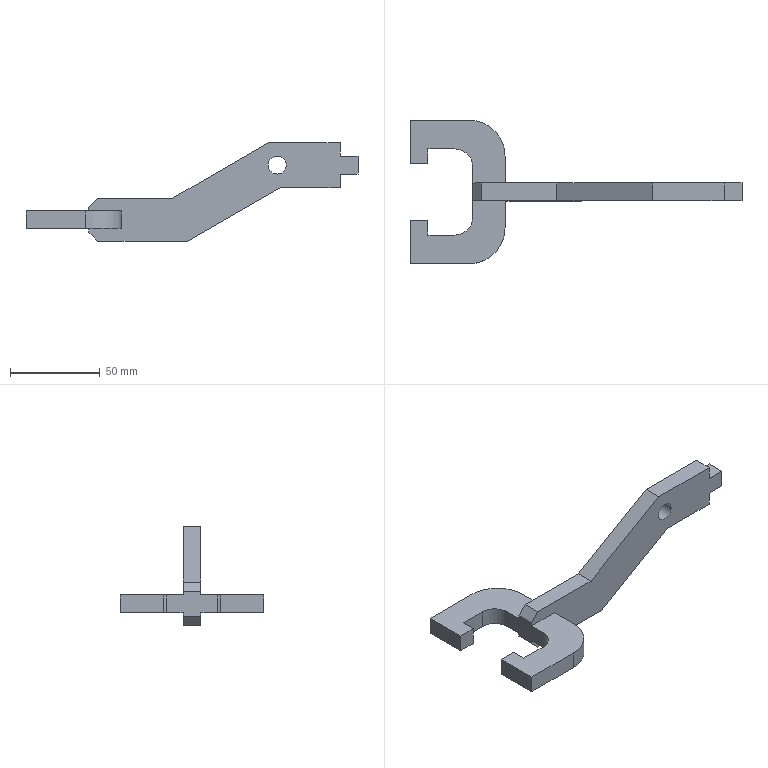Part | NX | features DATUM_CSYS 2, EXTRUDE 2, SKETCH 2, EXTRACT_DATUM_PLANE 1, LINKED_FACE 1 | 1 solid | 37 faces | box 185 x 80 x 55 mm | volume 60646 mm3 | plane 32 | cylinder 5 | commonest cylinder face diameters 20 x2 40 x2 10 x1
STEP:
#1=CARTESIAN_POINT('',(30.,5.,5.));
#2=VERTEX_POINT('',#1);
#3=CARTESIAN_POINT('',(30.,5.,7.));
#4=VERTEX_POINT('',#3);
#5=CARTESIAN_POINT('',(30.,5.,5.));
#6=DIRECTION('',(0.,0.,1.));
#7=VECTOR('',#6,1000.);
#8=LINE('',#5,#7);
#9=EDGE_CURVE('',#2,#4,#8,.T.);
#10=ORIENTED_EDGE('',*,*,#9,.F.);
#11=CARTESIAN_POINT('',(30.,14.,5.));
#12=VERTEX_POINT('',#11);
#13=CARTESIAN_POINT('',(30.,-14.,5.));
#14=DIRECTION('',(0.,1.,0.));
#15=VECTOR('',#14,1000.);
#16=LINE('',#13,#15);
#17=EDGE_CURVE('',#2,#12,#16,.T.);
#18=ORIENTED_EDGE('',*,*,#17,.T.);
#19=CARTESIAN_POINT('',(30.,14.,-5.));
#20=VERTEX_POINT('',#19);
#21=CARTESIAN_POINT('',(30.,14.,5.));
#22=DIRECTION('',(0.,0.,-1.));
#23=VECTOR('',#22,1000.);
#24=LINE('',#21,#23);
#25=EDGE_CURVE('',#12,#20,#24,.T.);
#26=ORIENTED_EDGE('',*,*,#25,.T.);
#27=CARTESIAN_POINT('',(30.,5.,-5.));
#28=VERTEX_POINT('',#27);
#29=CARTESIAN_POINT('',(30.,-14.,-5.));
#30=DIRECTION('',(0.,1.,0.));
#31=VECTOR('',#30,1000.);
#32=LINE('',#29,#31);
#33=EDGE_CURVE('',#28,#20,#32,.T.);
#34=ORIENTED_EDGE('',*,*,#33,.F.);
#35=CARTESIAN_POINT('',(30.,5.,-7.));
#36=VERTEX_POINT('',#35);
#37=CARTESIAN_POINT('',(30.,5.,-7.));
#38=DIRECTION('',(0.,0.,1.));
#39=VECTOR('',#38,1000.);
#40=LINE('',#37,#39);
#41=EDGE_CURVE('',#36,#28,#40,.T.);
#42=ORIENTED_EDGE('',*,*,#41,.F.);
#43=CARTESIAN_POINT('',(30.,-5.,-7.));
#44=VERTEX_POINT('',#43);
#45=CARTESIAN_POINT('',(30.,-5.,-7.));
#46=DIRECTION('',(0.,1.,0.));
#47=VECTOR('',#46,1000.);
#48=LINE('',#45,#47);
#49=EDGE_CURVE('',#44,#36,#48,.T.);
#50=ORIENTED_EDGE('',*,*,#49,.F.);
#51=CARTESIAN_POINT('',(30.,-5.,-5.));
#52=VERTEX_POINT('',#51);
#53=CARTESIAN_POINT('',(30.,-5.,-7.));
#54=DIRECTION('',(0.,0.,1.));
#55=VECTOR('',#54,1000.);
#56=LINE('',#53,#55);
#57=EDGE_CURVE('',#44,#52,#56,.T.);
#58=ORIENTED_EDGE('',*,*,#57,.T.);
#59=CARTESIAN_POINT('',(30.,-14.,-5.));
#60=VERTEX_POINT('',#59);
#61=CARTESIAN_POINT('',(30.,-14.,-5.));
#62=DIRECTION('',(0.,1.,0.));
#63=VECTOR('',#62,1000.);
#64=LINE('',#61,#63);
#65=EDGE_CURVE('',#60,#52,#64,.T.);
#66=ORIENTED_EDGE('',*,*,#65,.F.);
#67=CARTESIAN_POINT('',(30.,-14.,5.));
#68=VERTEX_POINT('',#67);
#69=CARTESIAN_POINT('',(30.,-14.,5.));
#70=DIRECTION('',(0.,0.,-1.));
#71=VECTOR('',#70,1000.);
#72=LINE('',#69,#71);
#73=EDGE_CURVE('',#68,#60,#72,.T.);
#74=ORIENTED_EDGE('',*,*,#73,.F.);
#75=CARTESIAN_POINT('',(30.,-5.,5.));
#76=VERTEX_POINT('',#75);
#77=CARTESIAN_POINT('',(30.,-14.,5.));
#78=DIRECTION('',(0.,1.,0.));
#79=VECTOR('',#78,1000.);
#80=LINE('',#77,#79);
#81=EDGE_CURVE('',#68,#76,#80,.T.);
#82=ORIENTED_EDGE('',*,*,#81,.T.);
#83=CARTESIAN_POINT('',(30.,-5.,7.));
#84=VERTEX_POINT('',#83);
#85=CARTESIAN_POINT('',(30.,-5.,5.));
#86=DIRECTION('',(0.,0.,1.));
#87=VECTOR('',#86,1000.);
#88=LINE('',#85,#87);
#89=EDGE_CURVE('',#76,#84,#88,.T.);
#90=ORIENTED_EDGE('',*,*,#89,.T.);
#91=CARTESIAN_POINT('',(30.,-5.,7.));
#92=DIRECTION('',(0.,1.,0.));
#93=VECTOR('',#92,1000.);
#94=LINE('',#91,#93);
#95=EDGE_CURVE('',#84,#4,#94,.T.);
#96=ORIENTED_EDGE('',*,*,#95,.T.);
#97=EDGE_LOOP('',(#10,#18,#26,#34,#42,#50,#58,#66,#74,#82,#90,#96));
#98=FACE_BOUND('',#97,.T.);
#99=CARTESIAN_POINT('',(30.,-5.,5.));
#100=DIRECTION('',(-1.,0.,0.));
#101=DIRECTION('',(0.,0.,1.));
#102=AXIS2_PLACEMENT_3D('',#99,#100,#101);
#103=PLANE('',#102);
#104=ADVANCED_FACE('',(#98),#103,.T.);
#105=CARTESIAN_POINT('',(35.016,5.,12.016));
#106=VERTEX_POINT('',#105);
#107=CARTESIAN_POINT('',(30.,5.,7.));
#108=DIRECTION('',(0.7071,0.,0.7071));
#109=VECTOR('',#108,1000.);
#110=LINE('',#107,#109);
#111=EDGE_CURVE('',#4,#106,#110,.T.);
#112=ORIENTED_EDGE('',*,*,#111,.F.);
#113=ORIENTED_EDGE('',*,*,#95,.F.);
#114=CARTESIAN_POINT('',(35.016,-5.,12.016));
#115=VERTEX_POINT('',#114);
#116=CARTESIAN_POINT('',(30.,-5.,7.));
#117=DIRECTION('',(0.7071,0.,0.7071));
#118=VECTOR('',#117,1000.);
#119=LINE('',#116,#118);
#120=EDGE_CURVE('',#84,#115,#119,.T.);
#121=ORIENTED_EDGE('',*,*,#120,.T.);
#122=CARTESIAN_POINT('',(35.016,-5.,12.016));
#123=DIRECTION('',(0.,1.,0.));
#124=VECTOR('',#123,1000.);
#125=LINE('',#122,#124);
#126=EDGE_CURVE('',#115,#106,#125,.T.);
#127=ORIENTED_EDGE('',*,*,#126,.T.);
#128=EDGE_LOOP('',(#112,#113,#121,#127));
#129=FACE_BOUND('',#128,.T.);
#130=CARTESIAN_POINT('',(30.,-5.,7.));
#131=DIRECTION('',(-0.7071,0.,0.7071));
#132=DIRECTION('',(0.7071,0.,0.7071));
#133=AXIS2_PLACEMENT_3D('',#130,#131,#132);
#134=PLANE('',#133);
#135=ADVANCED_FACE('',(#129),#134,.T.);
#136=CARTESIAN_POINT('',(76.823,5.,12.146));
#137=VERTEX_POINT('',#136);
#138=CARTESIAN_POINT('',(35.016,5.,12.016));
#139=DIRECTION('',(1.,0.,0.003125));
#140=VECTOR('',#139,1000.);
#141=LINE('',#138,#140);
#142=EDGE_CURVE('',#106,#137,#141,.T.);
#143=ORIENTED_EDGE('',*,*,#142,.F.);
#144=ORIENTED_EDGE('',*,*,#126,.F.);
#145=CARTESIAN_POINT('',(76.823,-5.,12.146));
#146=VERTEX_POINT('',#145);
#147=CARTESIAN_POINT('',(35.016,-5.,12.016));
#148=DIRECTION('',(1.,0.,0.003125));
#149=VECTOR('',#148,1000.);
#150=LINE('',#147,#149);
#151=EDGE_CURVE('',#115,#146,#150,.T.);
#152=ORIENTED_EDGE('',*,*,#151,.T.);
#153=CARTESIAN_POINT('',(76.823,-5.,12.146));
#154=DIRECTION('',(0.,1.,0.));
#155=VECTOR('',#154,1000.);
#156=LINE('',#153,#155);
#157=EDGE_CURVE('',#146,#137,#156,.T.);
#158=ORIENTED_EDGE('',*,*,#157,.T.);
#159=EDGE_LOOP('',(#143,#144,#152,#158));
#160=FACE_BOUND('',#159,.T.);
#161=CARTESIAN_POINT('',(35.016,-5.,12.016));
#162=DIRECTION('',(-0.003125,0.,1.));
#163=DIRECTION('',(1.,0.,0.003125));
#164=AXIS2_PLACEMENT_3D('',#161,#162,#163);
#165=PLANE('',#164);
#166=ADVANCED_FACE('',(#160),#165,.T.);
#167=CARTESIAN_POINT('',(130.263,5.,43.));
#168=VERTEX_POINT('',#167);
#169=CARTESIAN_POINT('',(76.823,5.,12.146));
#170=DIRECTION('',(0.866,0.,0.5));
#171=VECTOR('',#170,1000.);
#172=LINE('',#169,#171);
#173=EDGE_CURVE('',#137,#168,#172,.T.);
#174=ORIENTED_EDGE('',*,*,#173,.F.);
#175=ORIENTED_EDGE('',*,*,#157,.F.);
#176=CARTESIAN_POINT('',(130.263,-5.,43.));
#177=VERTEX_POINT('',#176);
#178=CARTESIAN_POINT('',(76.823,-5.,12.146));
#179=DIRECTION('',(0.866,0.,0.5));
#180=VECTOR('',#179,1000.);
#181=LINE('',#178,#180);
#182=EDGE_CURVE('',#146,#177,#181,.T.);
#183=ORIENTED_EDGE('',*,*,#182,.T.);
#184=CARTESIAN_POINT('',(130.263,-5.,43.));
#185=DIRECTION('',(0.,1.,0.));
#186=VECTOR('',#185,1000.);
#187=LINE('',#184,#186);
#188=EDGE_CURVE('',#177,#168,#187,.T.);
#189=ORIENTED_EDGE('',*,*,#188,.T.);
#190=EDGE_LOOP('',(#174,#175,#183,#189));
#191=FACE_BOUND('',#190,.T.);
#192=CARTESIAN_POINT('',(76.823,-5.,12.146));
#193=DIRECTION('',(-0.5,0.,0.866));
#194=DIRECTION('',(0.866,0.,0.5));
#195=AXIS2_PLACEMENT_3D('',#192,#193,#194);
#196=PLANE('',#195);
#197=ADVANCED_FACE('',(#191),#196,.T.);
#198=CARTESIAN_POINT('',(170.,5.,43.));
#199=VERTEX_POINT('',#198);
#200=CARTESIAN_POINT('',(130.263,5.,43.));
#201=DIRECTION('',(1.,0.,0.));
#202=VECTOR('',#201,1000.);
#203=LINE('',#200,#202);
#204=EDGE_CURVE('',#168,#199,#203,.T.);
#205=ORIENTED_EDGE('',*,*,#204,.F.);
#206=ORIENTED_EDGE('',*,*,#188,.F.);
#207=CARTESIAN_POINT('',(170.,-5.,43.));
#208=VERTEX_POINT('',#207);
#209=CARTESIAN_POINT('',(130.263,-5.,43.));
#210=DIRECTION('',(1.,0.,0.));
#211=VECTOR('',#210,1000.);
#212=LINE('',#209,#211);
#213=EDGE_CURVE('',#177,#208,#212,.T.);
#214=ORIENTED_EDGE('',*,*,#213,.T.);
#215=CARTESIAN_POINT('',(170.,-5.,43.));
#216=DIRECTION('',(0.,1.,0.));
#217=VECTOR('',#216,1000.);
#218=LINE('',#215,#217);
#219=EDGE_CURVE('',#208,#199,#218,.T.);
#220=ORIENTED_EDGE('',*,*,#219,.T.);
#221=EDGE_LOOP('',(#205,#206,#214,#220));
#222=FACE_BOUND('',#221,.T.);
#223=CARTESIAN_POINT('',(130.263,-5.,43.));
#224=DIRECTION('',(0.,0.,1.));
#225=DIRECTION('',(1.,0.,0.));
#226=AXIS2_PLACEMENT_3D('',#223,#224,#225);
#227=PLANE('',#226);
#228=ADVANCED_FACE('',(#222),#227,.T.);
#229=CARTESIAN_POINT('',(170.,5.,35.5));
#230=VERTEX_POINT('',#229);
#231=CARTESIAN_POINT('',(170.,5.,43.));
#232=DIRECTION('',(0.,0.,-1.));
#233=VECTOR('',#232,1000.);
#234=LINE('',#231,#233);
#235=EDGE_CURVE('',#199,#230,#234,.T.);
#236=ORIENTED_EDGE('',*,*,#235,.F.);
#237=ORIENTED_EDGE('',*,*,#219,.F.);
#238=CARTESIAN_POINT('',(170.,-5.,35.5));
#239=VERTEX_POINT('',#238);
#240=CARTESIAN_POINT('',(170.,-5.,43.));
#241=DIRECTION('',(0.,0.,-1.));
#242=VECTOR('',#241,1000.);
#243=LINE('',#240,#242);
#244=EDGE_CURVE('',#208,#239,#243,.T.);
#245=ORIENTED_EDGE('',*,*,#244,.T.);
#246=CARTESIAN_POINT('',(170.,-5.,35.5));
#247=DIRECTION('',(0.,1.,0.));
#248=VECTOR('',#247,1000.);
#249=LINE('',#246,#248);
#250=EDGE_CURVE('',#239,#230,#249,.T.);
#251=ORIENTED_EDGE('',*,*,#250,.T.);
#252=EDGE_LOOP('',(#236,#237,#245,#251));
#253=FACE_BOUND('',#252,.T.);
#254=CARTESIAN_POINT('',(170.,-5.,43.));
#255=DIRECTION('',(1.,0.,0.));
#256=DIRECTION('',(0.,0.,-1.));
#257=AXIS2_PLACEMENT_3D('',#254,#255,#256);
#258=PLANE('',#257);
#259=ADVANCED_FACE('',(#253),#258,.T.);
#260=CARTESIAN_POINT('',(180.,5.,35.5));
#261=VERTEX_POINT('',#260);
#262=CARTESIAN_POINT('',(170.,5.,35.5));
#263=DIRECTION('',(1.,0.,0.));
#264=VECTOR('',#263,1000.);
#265=LINE('',#262,#264);
#266=EDGE_CURVE('',#230,#261,#265,.T.);
#267=ORIENTED_EDGE('',*,*,#266,.F.);
#268=ORIENTED_EDGE('',*,*,#250,.F.);
#269=CARTESIAN_POINT('',(180.,-5.,35.5));
#270=VERTEX_POINT('',#269);
#271=CARTESIAN_POINT('',(170.,-5.,35.5));
#272=DIRECTION('',(1.,0.,0.));
#273=VECTOR('',#272,1000.);
#274=LINE('',#271,#273);
#275=EDGE_CURVE('',#239,#270,#274,.T.);
#276=ORIENTED_EDGE('',*,*,#275,.T.);
#277=CARTESIAN_POINT('',(180.,-5.,35.5));
#278=DIRECTION('',(0.,1.,0.));
#279=VECTOR('',#278,1000.);
#280=LINE('',#277,#279);
#281=EDGE_CURVE('',#270,#261,#280,.T.);
#282=ORIENTED_EDGE('',*,*,#281,.T.);
#283=EDGE_LOOP('',(#267,#268,#276,#282));
#284=FACE_BOUND('',#283,.T.);
#285=CARTESIAN_POINT('',(170.,-5.,35.5));
#286=DIRECTION('',(0.,0.,1.));
#287=DIRECTION('',(1.,0.,0.));
#288=AXIS2_PLACEMENT_3D('',#285,#286,#287);
#289=PLANE('',#288);
#290=ADVANCED_FACE('',(#284),#289,.T.);
#291=CARTESIAN_POINT('',(180.,5.,25.5));
#292=VERTEX_POINT('',#291);
#293=CARTESIAN_POINT('',(180.,5.,35.5));
#294=DIRECTION('',(0.,0.,-1.));
#295=VECTOR('',#294,1000.);
#296=LINE('',#293,#295);
#297=EDGE_CURVE('',#261,#292,#296,.T.);
#298=ORIENTED_EDGE('',*,*,#297,.F.);
#299=ORIENTED_EDGE('',*,*,#281,.F.);
#300=CARTESIAN_POINT('',(180.,-5.,25.5));
#301=VERTEX_POINT('',#300);
#302=CARTESIAN_POINT('',(180.,-5.,35.5));
#303=DIRECTION('',(0.,0.,-1.));
#304=VECTOR('',#303,1000.);
#305=LINE('',#302,#304);
#306=EDGE_CURVE('',#270,#301,#305,.T.);
#307=ORIENTED_EDGE('',*,*,#306,.T.);
#308=CARTESIAN_POINT('',(180.,-5.,25.5));
#309=DIRECTION('',(0.,1.,0.));
#310=VECTOR('',#309,1000.);
#311=LINE('',#308,#310);
#312=EDGE_CURVE('',#301,#292,#311,.T.);
#313=ORIENTED_EDGE('',*,*,#312,.T.);
#314=EDGE_LOOP('',(#298,#299,#307,#313));
#315=FACE_BOUND('',#314,.T.);
#316=CARTESIAN_POINT('',(180.,-5.,35.5));
#317=DIRECTION('',(1.,0.,0.));
#318=DIRECTION('',(0.,0.,-1.));
#319=AXIS2_PLACEMENT_3D('',#316,#317,#318);
#320=PLANE('',#319);
#321=ADVANCED_FACE('',(#315),#320,.T.);
#322=CARTESIAN_POINT('',(170.,5.,25.5));
#323=VERTEX_POINT('',#322);
#324=CARTESIAN_POINT('',(180.,5.,25.5));
#325=DIRECTION('',(-1.,0.,0.));
#326=VECTOR('',#325,1000.);
#327=LINE('',#324,#326);
#328=EDGE_CURVE('',#292,#323,#327,.T.);
#329=ORIENTED_EDGE('',*,*,#328,.F.);
#330=ORIENTED_EDGE('',*,*,#312,.F.);
#331=CARTESIAN_POINT('',(170.,-5.,25.5));
#332=VERTEX_POINT('',#331);
#333=CARTESIAN_POINT('',(180.,-5.,25.5));
#334=DIRECTION('',(-1.,0.,0.));
#335=VECTOR('',#334,1000.);
#336=LINE('',#333,#335);
#337=EDGE_CURVE('',#301,#332,#336,.T.);
#338=ORIENTED_EDGE('',*,*,#337,.T.);
#339=CARTESIAN_POINT('',(170.,-5.,25.5));
#340=DIRECTION('',(0.,1.,0.));
#341=VECTOR('',#340,1000.);
#342=LINE('',#339,#341);
#343=EDGE_CURVE('',#332,#323,#342,.T.);
#344=ORIENTED_EDGE('',*,*,#343,.T.);
#345=EDGE_LOOP('',(#329,#330,#338,#344));
#346=FACE_BOUND('',#345,.T.);
#347=CARTESIAN_POINT('',(180.,-5.,25.5));
#348=DIRECTION('',(0.,0.,-1.));
#349=DIRECTION('',(-1.,0.,0.));
#350=AXIS2_PLACEMENT_3D('',#347,#348,#349);
#351=PLANE('',#350);
#352=ADVANCED_FACE('',(#346),#351,.T.);
#353=CARTESIAN_POINT('',(170.,5.,18.));
#354=VERTEX_POINT('',#353);
#355=CARTESIAN_POINT('',(170.,5.,25.5));
#356=DIRECTION('',(0.,0.,-1.));
#357=VECTOR('',#356,1000.);
#358=LINE('',#355,#357);
#359=EDGE_CURVE('',#323,#354,#358,.T.);
#360=ORIENTED_EDGE('',*,*,#359,.F.);
#361=ORIENTED_EDGE('',*,*,#343,.F.);
#362=CARTESIAN_POINT('',(170.,-5.,18.));
#363=VERTEX_POINT('',#362);
#364=CARTESIAN_POINT('',(170.,-5.,25.5));
#365=DIRECTION('',(0.,0.,-1.));
#366=VECTOR('',#365,1000.);
#367=LINE('',#364,#366);
#368=EDGE_CURVE('',#332,#363,#367,.T.);
#369=ORIENTED_EDGE('',*,*,#368,.T.);
#370=CARTESIAN_POINT('',(170.,-5.,18.));
#371=DIRECTION('',(0.,1.,0.));
#372=VECTOR('',#371,1000.);
#373=LINE('',#370,#372);
#374=EDGE_CURVE('',#363,#354,#373,.T.);
#375=ORIENTED_EDGE('',*,*,#374,.T.);
#376=EDGE_LOOP('',(#360,#361,#369,#375));
#377=FACE_BOUND('',#376,.T.);
#378=CARTESIAN_POINT('',(170.,-5.,25.5));
#379=DIRECTION('',(1.,0.,0.));
#380=DIRECTION('',(0.,0.,-1.));
#381=AXIS2_PLACEMENT_3D('',#378,#379,#380);
#382=PLANE('',#381);
#383=ADVANCED_FACE('',(#377),#382,.T.);
#384=CARTESIAN_POINT('',(136.962,5.,18.));
#385=VERTEX_POINT('',#384);
#386=CARTESIAN_POINT('',(170.,5.,18.));
#387=DIRECTION('',(-1.,0.,0.));
#388=VECTOR('',#387,1000.);
#389=LINE('',#386,#388);
#390=EDGE_CURVE('',#354,#385,#389,.T.);
#391=ORIENTED_EDGE('',*,*,#390,.F.);
#392=ORIENTED_EDGE('',*,*,#374,.F.);
#393=CARTESIAN_POINT('',(136.962,-5.,18.));
#394=VERTEX_POINT('',#393);
#395=CARTESIAN_POINT('',(170.,-5.,18.));
#396=DIRECTION('',(-1.,0.,0.));
#397=VECTOR('',#396,1000.);
#398=LINE('',#395,#397);
#399=EDGE_CURVE('',#363,#394,#398,.T.);
#400=ORIENTED_EDGE('',*,*,#399,.T.);
#401=CARTESIAN_POINT('',(136.962,-5.,18.));
#402=DIRECTION('',(0.,1.,0.));
#403=VECTOR('',#402,1000.);
#404=LINE('',#401,#403);
#405=EDGE_CURVE('',#394,#385,#404,.T.);
#406=ORIENTED_EDGE('',*,*,#405,.T.);
#407=EDGE_LOOP('',(#391,#392,#400,#406));
#408=FACE_BOUND('',#407,.T.);
#409=CARTESIAN_POINT('',(170.,-5.,18.));
#410=DIRECTION('',(0.,0.,-1.));
#411=DIRECTION('',(-1.,0.,0.));
#412=AXIS2_PLACEMENT_3D('',#409,#410,#411);
#413=PLANE('',#412);
#414=ADVANCED_FACE('',(#408),#413,.T.);
#415=CARTESIAN_POINT('',(85.,5.,-12.));
#416=VERTEX_POINT('',#415);
#417=CARTESIAN_POINT('',(136.962,5.,18.));
#418=DIRECTION('',(-0.866,0.,-0.5));
#419=VECTOR('',#418,1000.);
#420=LINE('',#417,#419);
#421=EDGE_CURVE('',#385,#416,#420,.T.);
#422=ORIENTED_EDGE('',*,*,#421,.F.);
#423=ORIENTED_EDGE('',*,*,#405,.F.);
#424=CARTESIAN_POINT('',(85.,-5.,-12.));
#425=VERTEX_POINT('',#424);
#426=CARTESIAN_POINT('',(136.962,-5.,18.));
#427=DIRECTION('',(-0.866,0.,-0.5));
#428=VECTOR('',#427,1000.);
#429=LINE('',#426,#428);
#430=EDGE_CURVE('',#394,#425,#429,.T.);
#431=ORIENTED_EDGE('',*,*,#430,.T.);
#432=CARTESIAN_POINT('',(85.,-5.,-12.));
#433=DIRECTION('',(0.,1.,0.));
#434=VECTOR('',#433,1000.);
#435=LINE('',#432,#434);
#436=EDGE_CURVE('',#425,#416,#435,.T.);
#437=ORIENTED_EDGE('',*,*,#436,.T.);
#438=EDGE_LOOP('',(#422,#423,#431,#437));
#439=FACE_BOUND('',#438,.T.);
#440=CARTESIAN_POINT('',(136.962,-5.,18.));
#441=DIRECTION('',(0.5,0.,-0.866));
#442=DIRECTION('',(-0.866,0.,-0.5));
#443=AXIS2_PLACEMENT_3D('',#440,#441,#442);
#444=PLANE('',#443);
#445=ADVANCED_FACE('',(#439),#444,.T.);
#446=CARTESIAN_POINT('',(35.,5.,-12.));
#447=VERTEX_POINT('',#446);
#448=CARTESIAN_POINT('',(85.,5.,-12.));
#449=DIRECTION('',(-1.,0.,0.));
#450=VECTOR('',#449,1000.);
#451=LINE('',#448,#450);
#452=EDGE_CURVE('',#416,#447,#451,.T.);
#453=ORIENTED_EDGE('',*,*,#452,.F.);
#454=ORIENTED_EDGE('',*,*,#436,.F.);
#455=CARTESIAN_POINT('',(35.,-5.,-12.));
#456=VERTEX_POINT('',#455);
#457=CARTESIAN_POINT('',(85.,-5.,-12.));
#458=DIRECTION('',(-1.,0.,0.));
#459=VECTOR('',#458,1000.);
#460=LINE('',#457,#459);
#461=EDGE_CURVE('',#425,#456,#460,.T.);
#462=ORIENTED_EDGE('',*,*,#461,.T.);
#463=CARTESIAN_POINT('',(35.,-5.,-12.));
#464=DIRECTION('',(0.,1.,0.));
#465=VECTOR('',#464,1000.);
#466=LINE('',#463,#465);
#467=EDGE_CURVE('',#456,#447,#466,.T.);
#468=ORIENTED_EDGE('',*,*,#467,.T.);
#469=EDGE_LOOP('',(#453,#454,#462,#468));
#470=FACE_BOUND('',#469,.T.);
#471=CARTESIAN_POINT('',(85.,-5.,-12.));
#472=DIRECTION('',(0.,0.,-1.));
#473=DIRECTION('',(-1.,0.,0.));
#474=AXIS2_PLACEMENT_3D('',#471,#472,#473);
#475=PLANE('',#474);
#476=ADVANCED_FACE('',(#470),#475,.T.);
#477=CARTESIAN_POINT('',(35.,5.,-12.));
#478=DIRECTION('',(-0.7071,0.,0.7071));
#479=VECTOR('',#478,1000.);
#480=LINE('',#477,#479);
#481=EDGE_CURVE('',#447,#36,#480,.T.);
#482=ORIENTED_EDGE('',*,*,#481,.F.);
#483=ORIENTED_EDGE('',*,*,#467,.F.);
#484=CARTESIAN_POINT('',(35.,-5.,-12.));
#485=DIRECTION('',(-0.7071,0.,0.7071));
#486=VECTOR('',#485,1000.);
#487=LINE('',#484,#486);
#488=EDGE_CURVE('',#456,#44,#487,.T.);
#489=ORIENTED_EDGE('',*,*,#488,.T.);
#490=ORIENTED_EDGE('',*,*,#49,.T.);
#491=EDGE_LOOP('',(#482,#483,#489,#490));
#492=FACE_BOUND('',#491,.T.);
#493=CARTESIAN_POINT('',(35.,-5.,-12.));
#494=DIRECTION('',(-0.7071,0.,-0.7071));
#495=DIRECTION('',(-0.7071,0.,0.7071));
#496=AXIS2_PLACEMENT_3D('',#493,#494,#495);
#497=PLANE('',#496);
#498=ADVANCED_FACE('',(#492),#497,.T.);
#499=CARTESIAN_POINT('',(135.,5.,25.5));
#500=VERTEX_POINT('',#499);
#501=CARTESIAN_POINT('',(135.,5.,30.5));
#502=DIRECTION('',(0.,-1.,0.));
#503=DIRECTION('',(0.,0.,-1.));
#504=AXIS2_PLACEMENT_3D('',#501,#502,#503);
#505=CIRCLE('',#504,5.);
#506=EDGE_CURVE('',#500,#500,#505,.T.);
#507=ORIENTED_EDGE('',*,*,#506,.F.);
#508=EDGE_LOOP('',(#507));
#509=FACE_BOUND('',#508,.T.);
#510=CARTESIAN_POINT('',(135.,-5.,35.5));
#511=VERTEX_POINT('',#510);
#512=CARTESIAN_POINT('',(135.,-5.,30.5));
#513=DIRECTION('',(0.,-1.,0.));
#514=DIRECTION('',(0.,0.,1.));
#515=AXIS2_PLACEMENT_3D('',#512,#513,#514);
#516=CIRCLE('',#515,5.);
#517=EDGE_CURVE('',#511,#511,#516,.T.);
#518=ORIENTED_EDGE('',*,*,#517,.T.);
#519=EDGE_LOOP('',(#518));
#520=FACE_BOUND('',#519,.T.);
#521=CARTESIAN_POINT('',(135.,-5.,30.5));
#522=DIRECTION('',(0.,1.,0.));
#523=DIRECTION('',(0.,0.,1.));
#524=AXIS2_PLACEMENT_3D('',#521,#522,#523);
#525=CYLINDRICAL_SURFACE('',#524,5.);
#526=ADVANCED_FACE('',(#509,#520),#525,.F.);
#527=ORIENTED_EDGE('',*,*,#57,.F.);
#528=ORIENTED_EDGE('',*,*,#488,.F.);
#529=ORIENTED_EDGE('',*,*,#461,.F.);
#530=ORIENTED_EDGE('',*,*,#430,.F.);
#531=ORIENTED_EDGE('',*,*,#399,.F.);
#532=ORIENTED_EDGE('',*,*,#368,.F.);
#533=ORIENTED_EDGE('',*,*,#337,.F.);
#534=ORIENTED_EDGE('',*,*,#306,.F.);
#535=ORIENTED_EDGE('',*,*,#275,.F.);
#536=ORIENTED_EDGE('',*,*,#244,.F.);
#537=ORIENTED_EDGE('',*,*,#213,.F.);
#538=ORIENTED_EDGE('',*,*,#182,.F.);
#539=ORIENTED_EDGE('',*,*,#151,.F.);
#540=ORIENTED_EDGE('',*,*,#120,.F.);
#541=ORIENTED_EDGE('',*,*,#89,.F.);
#542=CARTESIAN_POINT('',(48.,-5.,5.));
#543=VERTEX_POINT('',#542);
#544=CARTESIAN_POINT('',(48.,-5.,5.));
#545=DIRECTION('',(-1.,0.,0.));
#546=VECTOR('',#545,1000.);
#547=LINE('',#544,#546);
#548=EDGE_CURVE('',#543,#76,#547,.T.);
#549=ORIENTED_EDGE('',*,*,#548,.F.);
#550=CARTESIAN_POINT('',(48.,-5.,-5.));
#551=VERTEX_POINT('',#550);
#552=CARTESIAN_POINT('',(48.,-5.,-5.));
#553=DIRECTION('',(0.,0.,1.));
#554=VECTOR('',#553,1000.);
#555=LINE('',#552,#554);
#556=EDGE_CURVE('',#551,#543,#555,.T.);
#557=ORIENTED_EDGE('',*,*,#556,.F.);
#558=CARTESIAN_POINT('',(30.,-5.,-5.));
#559=DIRECTION('',(1.,0.,0.));
#560=VECTOR('',#559,1000.);
#561=LINE('',#558,#560);
#562=EDGE_CURVE('',#52,#551,#561,.T.);
#563=ORIENTED_EDGE('',*,*,#562,.F.);
#564=EDGE_LOOP('',(#527,#528,#529,#530,#531,#532,#533,#534,#535,#536,#537,#538,#539,#540,#541,#549,#557,#563));
#565=FACE_BOUND('',#564,.T.);
#566=ORIENTED_EDGE('',*,*,#517,.F.);
#567=EDGE_LOOP('',(#566));
#568=FACE_BOUND('',#567,.T.);
#569=CARTESIAN_POINT('',(135.,-5.,30.5));
#570=DIRECTION('',(0.,-1.,0.));
#571=DIRECTION('',(0.,0.,-1.));
#572=AXIS2_PLACEMENT_3D('',#569,#570,#571);
#573=PLANE('',#572);
#574=ADVANCED_FACE('',(#565,#568),#573,.T.);
#575=ORIENTED_EDGE('',*,*,#41,.T.);
#576=CARTESIAN_POINT('',(48.,5.,-5.));
#577=VERTEX_POINT('',#576);
#578=CARTESIAN_POINT('',(30.,5.,-5.));
#579=DIRECTION('',(1.,0.,0.));
#580=VECTOR('',#579,1000.);
#581=LINE('',#578,#580);
#582=EDGE_CURVE('',#28,#577,#581,.T.);
#583=ORIENTED_EDGE('',*,*,#582,.T.);
#584=CARTESIAN_POINT('',(48.,5.,5.));
#585=VERTEX_POINT('',#584);
#586=CARTESIAN_POINT('',(48.,5.,-5.));
#587=DIRECTION('',(0.,0.,1.));
#588=VECTOR('',#587,1000.);
#589=LINE('',#586,#588);
#590=EDGE_CURVE('',#577,#585,#589,.T.);
#591=ORIENTED_EDGE('',*,*,#590,.T.);
#592=CARTESIAN_POINT('',(48.,5.,5.));
#593=DIRECTION('',(-1.,0.,0.));
#594=VECTOR('',#593,1000.);
#595=LINE('',#592,#594);
#596=EDGE_CURVE('',#585,#2,#595,.T.);
#597=ORIENTED_EDGE('',*,*,#596,.T.);
#598=ORIENTED_EDGE('',*,*,#9,.T.);
#599=ORIENTED_EDGE('',*,*,#111,.T.);
#600=ORIENTED_EDGE('',*,*,#142,.T.);
#601=ORIENTED_EDGE('',*,*,#173,.T.);
#602=ORIENTED_EDGE('',*,*,#204,.T.);
#603=ORIENTED_EDGE('',*,*,#235,.T.);
#604=ORIENTED_EDGE('',*,*,#266,.T.);
#605=ORIENTED_EDGE('',*,*,#297,.T.);
#606=ORIENTED_EDGE('',*,*,#328,.T.);
#607=ORIENTED_EDGE('',*,*,#359,.T.);
#608=ORIENTED_EDGE('',*,*,#390,.T.);
#609=ORIENTED_EDGE('',*,*,#421,.T.);
#610=ORIENTED_EDGE('',*,*,#452,.T.);
#611=ORIENTED_EDGE('',*,*,#481,.T.);
#612=EDGE_LOOP('',(#575,#583,#591,#597,#598,#599,#600,#601,#602,#603,#604,#605,#606,#607,#608,#609,#610,#611));
#613=FACE_BOUND('',#612,.T.);
#614=ORIENTED_EDGE('',*,*,#506,.T.);
#615=EDGE_LOOP('',(#614));
#616=FACE_BOUND('',#615,.T.);
#617=CARTESIAN_POINT('',(135.,5.,30.5));
#618=DIRECTION('',(0.,-1.,0.));
#619=DIRECTION('',(0.,0.,-1.));
#620=AXIS2_PLACEMENT_3D('',#617,#618,#619);
#621=PLANE('',#620);
#622=ADVANCED_FACE('',(#613,#616),#621,.F.);
#623=ORIENTED_EDGE('',*,*,#65,.T.);
#624=ORIENTED_EDGE('',*,*,#562,.T.);
#625=CARTESIAN_POINT('',(48.,-20.,-5.));
#626=VERTEX_POINT('',#625);
#627=CARTESIAN_POINT('',(48.,20.,-5.));
#628=DIRECTION('',(0.,-1.,0.));
#629=VECTOR('',#628,1000.);
#630=LINE('',#627,#629);
#631=EDGE_CURVE('',#551,#626,#630,.T.);
#632=ORIENTED_EDGE('',*,*,#631,.T.);
#633=CARTESIAN_POINT('',(28.,-40.,-5.));
#634=VERTEX_POINT('',#633);
#635=CARTESIAN_POINT('',(28.,-20.,-5.));
#636=DIRECTION('',(0.,0.,-1.));
#637=DIRECTION('',(1.,0.,0.));
#638=AXIS2_PLACEMENT_3D('',#635,#636,#637);
#639=CIRCLE('',#638,20.);
#640=EDGE_CURVE('',#626,#634,#639,.T.);
#641=ORIENTED_EDGE('',*,*,#640,.T.);
#642=CARTESIAN_POINT('',(-5.,-40.,-5.));
#643=VERTEX_POINT('',#642);
#644=CARTESIAN_POINT('',(-3.,-40.,-5.));
#645=DIRECTION('',(-1.,0.,0.));
#646=VECTOR('',#645,1000.);
#647=LINE('',#644,#646);
#648=EDGE_CURVE('',#634,#643,#647,.T.);
#649=ORIENTED_EDGE('',*,*,#648,.T.);
#650=CARTESIAN_POINT('',(-5.,-16.,-5.));
#651=VERTEX_POINT('',#650);
#652=CARTESIAN_POINT('',(-5.,-40.,-5.));
#653=DIRECTION('',(0.,1.,0.));
#654=VECTOR('',#653,1000.);
#655=LINE('',#652,#654);
#656=EDGE_CURVE('',#643,#651,#655,.T.);
#657=ORIENTED_EDGE('',*,*,#656,.T.);
#658=CARTESIAN_POINT('',(5.,-16.,-5.));
#659=VERTEX_POINT('',#658);
#660=CARTESIAN_POINT('',(3.,-16.,-5.));
#661=DIRECTION('',(1.,0.,0.));
#662=VECTOR('',#661,1000.);
#663=LINE('',#660,#662);
#664=EDGE_CURVE('',#651,#659,#663,.T.);
#665=ORIENTED_EDGE('',*,*,#664,.T.);
#666=CARTESIAN_POINT('',(5.,-24.,-5.));
#667=VERTEX_POINT('',#666);
#668=CARTESIAN_POINT('',(5.,-16.,-5.));
#669=DIRECTION('',(0.,-1.,0.));
#670=VECTOR('',#669,1000.);
#671=LINE('',#668,#670);
#672=EDGE_CURVE('',#659,#667,#671,.T.);
#673=ORIENTED_EDGE('',*,*,#672,.T.);
#674=CARTESIAN_POINT('',(20.,-24.,-5.));
#675=VERTEX_POINT('',#674);
#676=CARTESIAN_POINT('',(5.,-24.,-5.));
#677=DIRECTION('',(1.,0.,0.));
#678=VECTOR('',#677,1000.);
#679=LINE('',#676,#678);
#680=EDGE_CURVE('',#667,#675,#679,.T.);
#681=ORIENTED_EDGE('',*,*,#680,.T.);
#682=CARTESIAN_POINT('',(20.,-14.,-5.));
#683=DIRECTION('',(0.,0.,1.));
#684=DIRECTION('',(0.,-1.,0.));
#685=AXIS2_PLACEMENT_3D('',#682,#683,#684);
#686=CIRCLE('',#685,10.);
#687=EDGE_CURVE('',#675,#60,#686,.T.);
#688=ORIENTED_EDGE('',*,*,#687,.T.);
#689=EDGE_LOOP('',(#623,#624,#632,#641,#649,#657,#665,#673,#681,#688));
#690=FACE_BOUND('',#689,.T.);
#691=CARTESIAN_POINT('',(20.,-14.,-5.));
#692=DIRECTION('',(0.,0.,1.));
#693=DIRECTION('',(1.,0.,0.));
#694=AXIS2_PLACEMENT_3D('',#691,#692,#693);
#695=PLANE('',#694);
#696=ADVANCED_FACE('',(#690),#695,.F.);
#697=ORIENTED_EDGE('',*,*,#590,.F.);
#698=CARTESIAN_POINT('',(48.,20.,-5.));
#699=VERTEX_POINT('',#698);
#700=CARTESIAN_POINT('',(48.,20.,-5.));
#701=DIRECTION('',(0.,-1.,0.));
#702=VECTOR('',#701,1000.);
#703=LINE('',#700,#702);
#704=EDGE_CURVE('',#699,#577,#703,.T.);
#705=ORIENTED_EDGE('',*,*,#704,.F.);
#706=CARTESIAN_POINT('',(48.,20.,5.));
#707=VERTEX_POINT('',#706);
#708=CARTESIAN_POINT('',(48.,20.,5.));
#709=DIRECTION('',(0.,0.,-1.));
#710=VECTOR('',#709,1000.);
#711=LINE('',#708,#710);
#712=EDGE_CURVE('',#707,#699,#711,.T.);
#713=ORIENTED_EDGE('',*,*,#712,.F.);
#714=CARTESIAN_POINT('',(48.,20.,5.));
#715=DIRECTION('',(0.,-1.,0.));
#716=VECTOR('',#715,1000.);
#717=LINE('',#714,#716);
#718=EDGE_CURVE('',#707,#585,#717,.T.);
#719=ORIENTED_EDGE('',*,*,#718,.T.);
#720=EDGE_LOOP('',(#697,#705,#713,#719));
#721=FACE_BOUND('',#720,.T.);
#722=CARTESIAN_POINT('',(48.,20.,5.));
#723=DIRECTION('',(1.,0.,0.));
#724=DIRECTION('',(0.,0.,-1.));
#725=AXIS2_PLACEMENT_3D('',#722,#723,#724);
#726=PLANE('',#725);
#727=ADVANCED_FACE('',(#721),#726,.T.);
#728=ORIENTED_EDGE('',*,*,#596,.F.);
#729=ORIENTED_EDGE('',*,*,#718,.F.);
#730=CARTESIAN_POINT('',(28.,40.,5.));
#731=VERTEX_POINT('',#730);
#732=CARTESIAN_POINT('',(28.,20.,5.));
#733=DIRECTION('',(0.,0.,-1.));
#734=DIRECTION('',(0.,1.,0.));
#735=AXIS2_PLACEMENT_3D('',#732,#733,#734);
#736=CIRCLE('',#735,20.);
#737=EDGE_CURVE('',#731,#707,#736,.T.);
#738=ORIENTED_EDGE('',*,*,#737,.F.);
#739=CARTESIAN_POINT('',(-5.,40.,5.));
#740=VERTEX_POINT('',#739);
#741=CARTESIAN_POINT('',(-5.,40.,5.));
#742=DIRECTION('',(1.,0.,0.));
#743=VECTOR('',#742,1000.);
#744=LINE('',#741,#743);
#745=EDGE_CURVE('',#740,#731,#744,.T.);
#746=ORIENTED_EDGE('',*,*,#745,.F.);
#747=CARTESIAN_POINT('',(-5.,16.,5.));
#748=VERTEX_POINT('',#747);
#749=CARTESIAN_POINT('',(-5.,16.,5.));
#750=DIRECTION('',(0.,1.,0.));
#751=VECTOR('',#750,1000.);
#752=LINE('',#749,#751);
#753=EDGE_CURVE('',#748,#740,#752,.T.);
#754=ORIENTED_EDGE('',*,*,#753,.F.);
#755=CARTESIAN_POINT('',(5.,16.,5.));
#756=VERTEX_POINT('',#755);
#757=CARTESIAN_POINT('',(5.,16.,5.));
#758=DIRECTION('',(-1.,0.,0.));
#759=VECTOR('',#758,1000.);
#760=LINE('',#757,#759);
#761=EDGE_CURVE('',#756,#748,#760,.T.);
#762=ORIENTED_EDGE('',*,*,#761,.F.);
#763=CARTESIAN_POINT('',(5.,24.,5.));
#764=VERTEX_POINT('',#763);
#765=CARTESIAN_POINT('',(5.,24.,5.));
#766=DIRECTION('',(0.,-1.,0.));
#767=VECTOR('',#766,1000.);
#768=LINE('',#765,#767);
#769=EDGE_CURVE('',#764,#756,#768,.T.);
#770=ORIENTED_EDGE('',*,*,#769,.F.);
#771=CARTESIAN_POINT('',(20.,24.,5.));
#772=VERTEX_POINT('',#771);
#773=CARTESIAN_POINT('',(20.,24.,5.));
#774=DIRECTION('',(-1.,0.,0.));
#775=VECTOR('',#774,1000.);
#776=LINE('',#773,#775);
#777=EDGE_CURVE('',#772,#764,#776,.T.);
#778=ORIENTED_EDGE('',*,*,#777,.F.);
#779=CARTESIAN_POINT('',(20.,14.,5.));
#780=DIRECTION('',(0.,0.,1.));
#781=DIRECTION('',(1.,0.,0.));
#782=AXIS2_PLACEMENT_3D('',#779,#780,#781);
#783=CIRCLE('',#782,10.);
#784=EDGE_CURVE('',#12,#772,#783,.T.);
#785=ORIENTED_EDGE('',*,*,#784,.F.);
#786=ORIENTED_EDGE('',*,*,#17,.F.);
#787=EDGE_LOOP('',(#728,#729,#738,#746,#754,#762,#770,#778,#785,#786));
#788=FACE_BOUND('',#787,.T.);
#789=CARTESIAN_POINT('',(20.,-14.,5.));
#790=DIRECTION('',(0.,0.,1.));
#791=DIRECTION('',(1.,0.,0.));
#792=AXIS2_PLACEMENT_3D('',#789,#790,#791);
#793=PLANE('',#792);
#794=ADVANCED_FACE('',(#788),#793,.T.);
#795=ORIENTED_EDGE('',*,*,#656,.F.);
#796=CARTESIAN_POINT('',(-5.,-40.,5.));
#797=VERTEX_POINT('',#796);
#798=CARTESIAN_POINT('',(-5.,-40.,5.));
#799=DIRECTION('',(0.,0.,-1.));
#800=VECTOR('',#799,1000.);
#801=LINE('',#798,#800);
#802=EDGE_CURVE('',#797,#643,#801,.T.);
#803=ORIENTED_EDGE('',*,*,#802,.F.);
#804=CARTESIAN_POINT('',(-5.,-16.,5.));
#805=VERTEX_POINT('',#804);
#806=CARTESIAN_POINT('',(-5.,-40.,5.));
#807=DIRECTION('',(0.,1.,0.));
#808=VECTOR('',#807,1000.);
#809=LINE('',#806,#808);
#810=EDGE_CURVE('',#797,#805,#809,.T.);
#811=ORIENTED_EDGE('',*,*,#810,.T.);
#812=CARTESIAN_POINT('',(-5.,-16.,5.));
#813=DIRECTION('',(0.,0.,-1.));
#814=VECTOR('',#813,1000.);
#815=LINE('',#812,#814);
#816=EDGE_CURVE('',#805,#651,#815,.T.);
#817=ORIENTED_EDGE('',*,*,#816,.T.);
#818=EDGE_LOOP('',(#795,#803,#811,#817));
#819=FACE_BOUND('',#818,.T.);
#820=CARTESIAN_POINT('',(-5.,-40.,5.));
#821=DIRECTION('',(-1.,0.,0.));
#822=DIRECTION('',(0.,0.,1.));
#823=AXIS2_PLACEMENT_3D('',#820,#821,#822);
#824=PLANE('',#823);
#825=ADVANCED_FACE('',(#819),#824,.T.);
#826=ORIENTED_EDGE('',*,*,#664,.F.);
#827=ORIENTED_EDGE('',*,*,#816,.F.);
#828=CARTESIAN_POINT('',(5.,-16.,5.));
#829=VERTEX_POINT('',#828);
#830=CARTESIAN_POINT('',(-5.,-16.,5.));
#831=DIRECTION('',(1.,0.,0.));
#832=VECTOR('',#831,1000.);
#833=LINE('',#830,#832);
#834=EDGE_CURVE('',#805,#829,#833,.T.);
#835=ORIENTED_EDGE('',*,*,#834,.T.);
#836=CARTESIAN_POINT('',(5.,-16.,5.));
#837=DIRECTION('',(0.,0.,-1.));
#838=VECTOR('',#837,1000.);
#839=LINE('',#836,#838);
#840=EDGE_CURVE('',#829,#659,#839,.T.);
#841=ORIENTED_EDGE('',*,*,#840,.T.);
#842=EDGE_LOOP('',(#826,#827,#835,#841));
#843=FACE_BOUND('',#842,.T.);
#844=CARTESIAN_POINT('',(3.,-16.,5.));
#845=DIRECTION('',(0.,1.,0.));
#846=DIRECTION('',(0.,0.,1.));
#847=AXIS2_PLACEMENT_3D('',#844,#845,#846);
#848=PLANE('',#847);
#849=ADVANCED_FACE('',(#843),#848,.T.);
#850=ORIENTED_EDGE('',*,*,#672,.F.);
#851=ORIENTED_EDGE('',*,*,#840,.F.);
#852=CARTESIAN_POINT('',(5.,-24.,5.));
#853=VERTEX_POINT('',#852);
#854=CARTESIAN_POINT('',(5.,-16.,5.));
#855=DIRECTION('',(0.,-1.,0.));
#856=VECTOR('',#855,1000.);
#857=LINE('',#854,#856);
#858=EDGE_CURVE('',#829,#853,#857,.T.);
#859=ORIENTED_EDGE('',*,*,#858,.T.);
#860=CARTESIAN_POINT('',(5.,-24.,5.));
#861=DIRECTION('',(0.,0.,-1.));
#862=VECTOR('',#861,1000.);
#863=LINE('',#860,#862);
#864=EDGE_CURVE('',#853,#667,#863,.T.);
#865=ORIENTED_EDGE('',*,*,#864,.T.);
#866=EDGE_LOOP('',(#850,#851,#859,#865));
#867=FACE_BOUND('',#866,.T.);
#868=CARTESIAN_POINT('',(5.,-16.,5.));
#869=DIRECTION('',(1.,0.,0.));
#870=DIRECTION('',(0.,0.,-1.));
#871=AXIS2_PLACEMENT_3D('',#868,#869,#870);
#872=PLANE('',#871);
#873=ADVANCED_FACE('',(#867),#872,.T.);
#874=ORIENTED_EDGE('',*,*,#680,.F.);
#875=ORIENTED_EDGE('',*,*,#864,.F.);
#876=CARTESIAN_POINT('',(20.,-24.,5.));
#877=VERTEX_POINT('',#876);
#878=CARTESIAN_POINT('',(5.,-24.,5.));
#879=DIRECTION('',(1.,0.,0.));
#880=VECTOR('',#879,1000.);
#881=LINE('',#878,#880);
#882=EDGE_CURVE('',#853,#877,#881,.T.);
#883=ORIENTED_EDGE('',*,*,#882,.T.);
#884=CARTESIAN_POINT('',(20.,-24.,5.));
#885=DIRECTION('',(0.,0.,-1.));
#886=VECTOR('',#885,1000.);
#887=LINE('',#884,#886);
#888=EDGE_CURVE('',#877,#675,#887,.T.);
#889=ORIENTED_EDGE('',*,*,#888,.T.);
#890=EDGE_LOOP('',(#874,#875,#883,#889));
#891=FACE_BOUND('',#890,.T.);
#892=CARTESIAN_POINT('',(5.,-24.,5.));
#893=DIRECTION('',(0.,1.,0.));
#894=DIRECTION('',(0.,0.,1.));
#895=AXIS2_PLACEMENT_3D('',#892,#893,#894);
#896=PLANE('',#895);
#897=ADVANCED_FACE('',(#891),#896,.T.);
#898=ORIENTED_EDGE('',*,*,#687,.F.);
#899=ORIENTED_EDGE('',*,*,#888,.F.);
#900=CARTESIAN_POINT('',(20.,-14.,5.));
#901=DIRECTION('',(0.,0.,1.));
#902=DIRECTION('',(0.,-1.,0.));
#903=AXIS2_PLACEMENT_3D('',#900,#901,#902);
#904=CIRCLE('',#903,10.);
#905=EDGE_CURVE('',#877,#68,#904,.T.);
#906=ORIENTED_EDGE('',*,*,#905,.T.);
#907=ORIENTED_EDGE('',*,*,#73,.T.);
#908=EDGE_LOOP('',(#898,#899,#906,#907));
#909=FACE_BOUND('',#908,.T.);
#910=CARTESIAN_POINT('',(20.,-14.,5.));
#911=DIRECTION('',(0.,0.,-1.));
#912=DIRECTION('',(-1.,0.,0.));
#913=AXIS2_PLACEMENT_3D('',#910,#911,#912);
#914=CYLINDRICAL_SURFACE('',#913,10.);
#915=ADVANCED_FACE('',(#909),#914,.F.);
#916=CARTESIAN_POINT('',(20.,24.,-5.));
#917=VERTEX_POINT('',#916);
#918=CARTESIAN_POINT('',(20.,14.,-5.));
#919=DIRECTION('',(0.,0.,1.));
#920=DIRECTION('',(1.,0.,0.));
#921=AXIS2_PLACEMENT_3D('',#918,#919,#920);
#922=CIRCLE('',#921,10.);
#923=EDGE_CURVE('',#20,#917,#922,.T.);
#924=ORIENTED_EDGE('',*,*,#923,.F.);
#925=ORIENTED_EDGE('',*,*,#25,.F.);
#926=ORIENTED_EDGE('',*,*,#784,.T.);
#927=CARTESIAN_POINT('',(20.,24.,5.));
#928=DIRECTION('',(0.,0.,-1.));
#929=VECTOR('',#928,1000.);
#930=LINE('',#927,#929);
#931=EDGE_CURVE('',#772,#917,#930,.T.);
#932=ORIENTED_EDGE('',*,*,#931,.T.);
#933=EDGE_LOOP('',(#924,#925,#926,#932));
#934=FACE_BOUND('',#933,.T.);
#935=CARTESIAN_POINT('',(20.,14.,5.));
#936=DIRECTION('',(0.,0.,-1.));
#937=DIRECTION('',(-1.,0.,0.));
#938=AXIS2_PLACEMENT_3D('',#935,#936,#937);
#939=CYLINDRICAL_SURFACE('',#938,10.);
#940=ADVANCED_FACE('',(#934),#939,.F.);
#941=CARTESIAN_POINT('',(5.,24.,-5.));
#942=VERTEX_POINT('',#941);
#943=CARTESIAN_POINT('',(20.,24.,-5.));
#944=DIRECTION('',(-1.,0.,0.));
#945=VECTOR('',#944,1000.);
#946=LINE('',#943,#945);
#947=EDGE_CURVE('',#917,#942,#946,.T.);
#948=ORIENTED_EDGE('',*,*,#947,.F.);
#949=ORIENTED_EDGE('',*,*,#931,.F.);
#950=ORIENTED_EDGE('',*,*,#777,.T.);
#951=CARTESIAN_POINT('',(5.,24.,5.));
#952=DIRECTION('',(0.,0.,-1.));
#953=VECTOR('',#952,1000.);
#954=LINE('',#951,#953);
#955=EDGE_CURVE('',#764,#942,#954,.T.);
#956=ORIENTED_EDGE('',*,*,#955,.T.);
#957=EDGE_LOOP('',(#948,#949,#950,#956));
#958=FACE_BOUND('',#957,.T.);
#959=CARTESIAN_POINT('',(20.,24.,5.));
#960=DIRECTION('',(0.,-1.,0.));
#961=DIRECTION('',(0.,0.,-1.));
#962=AXIS2_PLACEMENT_3D('',#959,#960,#961);
#963=PLANE('',#962);
#964=ADVANCED_FACE('',(#958),#963,.T.);
#965=CARTESIAN_POINT('',(5.,16.,-5.));
#966=VERTEX_POINT('',#965);
#967=CARTESIAN_POINT('',(5.,24.,-5.));
#968=DIRECTION('',(0.,-1.,0.));
#969=VECTOR('',#968,1000.);
#970=LINE('',#967,#969);
#971=EDGE_CURVE('',#942,#966,#970,.T.);
#972=ORIENTED_EDGE('',*,*,#971,.F.);
#973=ORIENTED_EDGE('',*,*,#955,.F.);
#974=ORIENTED_EDGE('',*,*,#769,.T.);
#975=CARTESIAN_POINT('',(5.,16.,5.));
#976=DIRECTION('',(0.,0.,-1.));
#977=VECTOR('',#976,1000.);
#978=LINE('',#975,#977);
#979=EDGE_CURVE('',#756,#966,#978,.T.);
#980=ORIENTED_EDGE('',*,*,#979,.T.);
#981=EDGE_LOOP('',(#972,#973,#974,#980));
#982=FACE_BOUND('',#981,.T.);
#983=CARTESIAN_POINT('',(5.,24.,5.));
#984=DIRECTION('',(1.,0.,0.));
#985=DIRECTION('',(0.,0.,-1.));
#986=AXIS2_PLACEMENT_3D('',#983,#984,#985);
#987=PLANE('',#986);
#988=ADVANCED_FACE('',(#982),#987,.T.);
#989=CARTESIAN_POINT('',(-5.,16.,-5.));
#990=VERTEX_POINT('',#989);
#991=CARTESIAN_POINT('',(-3.,16.,-5.));
#992=DIRECTION('',(-1.,0.,0.));
#993=VECTOR('',#992,1000.);
#994=LINE('',#991,#993);
#995=EDGE_CURVE('',#966,#990,#994,.T.);
#996=ORIENTED_EDGE('',*,*,#995,.F.);
#997=ORIENTED_EDGE('',*,*,#979,.F.);
#998=ORIENTED_EDGE('',*,*,#761,.T.);
#999=CARTESIAN_POINT('',(-5.,16.,5.));
#1000=DIRECTION('',(0.,0.,-1.));
#1001=VECTOR('',#1000,1000.);
#1002=LINE('',#999,#1001);
#1003=EDGE_CURVE('',#748,#990,#1002,.T.);
#1004=ORIENTED_EDGE('',*,*,#1003,.T.);
#1005=EDGE_LOOP('',(#996,#997,#998,#1004));
#1006=FACE_BOUND('',#1005,.T.);
#1007=CARTESIAN_POINT('',(-3.,16.,5.));
#1008=DIRECTION('',(0.,-1.,0.));
#1009=DIRECTION('',(0.,0.,-1.));
#1010=AXIS2_PLACEMENT_3D('',#1007,#1008,#1009);
#1011=PLANE('',#1010);
#1012=ADVANCED_FACE('',(#1006),#1011,.T.);
#1013=CARTESIAN_POINT('',(-5.,40.,-5.));
#1014=VERTEX_POINT('',#1013);
#1015=CARTESIAN_POINT('',(-5.,16.,-5.));
#1016=DIRECTION('',(0.,1.,0.));
#1017=VECTOR('',#1016,1000.);
#1018=LINE('',#1015,#1017);
#1019=EDGE_CURVE('',#990,#1014,#1018,.T.);
#1020=ORIENTED_EDGE('',*,*,#1019,.F.);
#1021=ORIENTED_EDGE('',*,*,#1003,.F.);
#1022=ORIENTED_EDGE('',*,*,#753,.T.);
#1023=CARTESIAN_POINT('',(-5.,40.,5.));
#1024=DIRECTION('',(0.,0.,-1.));
#1025=VECTOR('',#1024,1000.);
#1026=LINE('',#1023,#1025);
#1027=EDGE_CURVE('',#740,#1014,#1026,.T.);
#1028=ORIENTED_EDGE('',*,*,#1027,.T.);
#1029=EDGE_LOOP('',(#1020,#1021,#1022,#1028));
#1030=FACE_BOUND('',#1029,.T.);
#1031=CARTESIAN_POINT('',(-5.,16.,5.));
#1032=DIRECTION('',(-1.,0.,0.));
#1033=DIRECTION('',(0.,0.,1.));
#1034=AXIS2_PLACEMENT_3D('',#1031,#1032,#1033);
#1035=PLANE('',#1034);
#1036=ADVANCED_FACE('',(#1030),#1035,.T.);
#1037=CARTESIAN_POINT('',(28.,40.,-5.));
#1038=VERTEX_POINT('',#1037);
#1039=CARTESIAN_POINT('',(-3.,40.,-5.));
#1040=DIRECTION('',(1.,0.,0.));
#1041=VECTOR('',#1040,1000.);
#1042=LINE('',#1039,#1041);
#1043=EDGE_CURVE('',#1014,#1038,#1042,.T.);
#1044=ORIENTED_EDGE('',*,*,#1043,.F.);
#1045=ORIENTED_EDGE('',*,*,#1027,.F.);
#1046=ORIENTED_EDGE('',*,*,#745,.T.);
#1047=CARTESIAN_POINT('',(28.,40.,5.));
#1048=DIRECTION('',(0.,0.,-1.));
#1049=VECTOR('',#1048,1000.);
#1050=LINE('',#1047,#1049);
#1051=EDGE_CURVE('',#731,#1038,#1050,.T.);
#1052=ORIENTED_EDGE('',*,*,#1051,.T.);
#1053=EDGE_LOOP('',(#1044,#1045,#1046,#1052));
#1054=FACE_BOUND('',#1053,.T.);
#1055=CARTESIAN_POINT('',(-3.,40.,5.));
#1056=DIRECTION('',(0.,1.,0.));
#1057=DIRECTION('',(0.,0.,1.));
#1058=AXIS2_PLACEMENT_3D('',#1055,#1056,#1057);
#1059=PLANE('',#1058);
#1060=ADVANCED_FACE('',(#1054),#1059,.T.);
#1061=CARTESIAN_POINT('',(28.,20.,-5.));
#1062=DIRECTION('',(0.,0.,-1.));
#1063=DIRECTION('',(0.,1.,0.));
#1064=AXIS2_PLACEMENT_3D('',#1061,#1062,#1063);
#1065=CIRCLE('',#1064,20.);
#1066=EDGE_CURVE('',#1038,#699,#1065,.T.);
#1067=ORIENTED_EDGE('',*,*,#1066,.F.);
#1068=ORIENTED_EDGE('',*,*,#1051,.F.);
#1069=ORIENTED_EDGE('',*,*,#737,.T.);
#1070=ORIENTED_EDGE('',*,*,#712,.T.);
#1071=EDGE_LOOP('',(#1067,#1068,#1069,#1070));
#1072=FACE_BOUND('',#1071,.T.);
#1073=CARTESIAN_POINT('',(28.,20.,5.));
#1074=DIRECTION('',(0.,0.,-1.));
#1075=DIRECTION('',(-1.,0.,0.));
#1076=AXIS2_PLACEMENT_3D('',#1073,#1074,#1075);
#1077=CYLINDRICAL_SURFACE('',#1076,20.);
#1078=ADVANCED_FACE('',(#1072),#1077,.T.);
#1079=ORIENTED_EDGE('',*,*,#631,.F.);
#1080=ORIENTED_EDGE('',*,*,#556,.T.);
#1081=CARTESIAN_POINT('',(48.,-20.,5.));
#1082=VERTEX_POINT('',#1081);
#1083=CARTESIAN_POINT('',(48.,20.,5.));
#1084=DIRECTION('',(0.,-1.,0.));
#1085=VECTOR('',#1084,1000.);
#1086=LINE('',#1083,#1085);
#1087=EDGE_CURVE('',#543,#1082,#1086,.T.);
#1088=ORIENTED_EDGE('',*,*,#1087,.T.);
#1089=CARTESIAN_POINT('',(48.,-20.,5.));
#1090=DIRECTION('',(0.,0.,-1.));
#1091=VECTOR('',#1090,1000.);
#1092=LINE('',#1089,#1091);
#1093=EDGE_CURVE('',#1082,#626,#1092,.T.);
#1094=ORIENTED_EDGE('',*,*,#1093,.T.);
#1095=EDGE_LOOP('',(#1079,#1080,#1088,#1094));
#1096=FACE_BOUND('',#1095,.T.);
#1097=CARTESIAN_POINT('',(48.,20.,5.));
#1098=DIRECTION('',(1.,0.,0.));
#1099=DIRECTION('',(0.,0.,-1.));
#1100=AXIS2_PLACEMENT_3D('',#1097,#1098,#1099);
#1101=PLANE('',#1100);
#1102=ADVANCED_FACE('',(#1096),#1101,.T.);
#1103=ORIENTED_EDGE('',*,*,#640,.F.);
#1104=ORIENTED_EDGE('',*,*,#1093,.F.);
#1105=CARTESIAN_POINT('',(28.,-40.,5.));
#1106=VERTEX_POINT('',#1105);
#1107=CARTESIAN_POINT('',(28.,-20.,5.));
#1108=DIRECTION('',(0.,0.,-1.));
#1109=DIRECTION('',(1.,0.,0.));
#1110=AXIS2_PLACEMENT_3D('',#1107,#1108,#1109);
#1111=CIRCLE('',#1110,20.);
#1112=EDGE_CURVE('',#1082,#1106,#1111,.T.);
#1113=ORIENTED_EDGE('',*,*,#1112,.T.);
#1114=CARTESIAN_POINT('',(28.,-40.,5.));
#1115=DIRECTION('',(0.,0.,-1.));
#1116=VECTOR('',#1115,1000.);
#1117=LINE('',#1114,#1116);
#1118=EDGE_CURVE('',#1106,#634,#1117,.T.);
#1119=ORIENTED_EDGE('',*,*,#1118,.T.);
#1120=EDGE_LOOP('',(#1103,#1104,#1113,#1119));
#1121=FACE_BOUND('',#1120,.T.);
#1122=CARTESIAN_POINT('',(28.,-20.,5.));
#1123=DIRECTION('',(0.,0.,-1.));
#1124=DIRECTION('',(-1.,0.,0.));
#1125=AXIS2_PLACEMENT_3D('',#1122,#1123,#1124);
#1126=CYLINDRICAL_SURFACE('',#1125,20.);
#1127=ADVANCED_FACE('',(#1121),#1126,.T.);
#1128=ORIENTED_EDGE('',*,*,#648,.F.);
#1129=ORIENTED_EDGE('',*,*,#1118,.F.);
#1130=CARTESIAN_POINT('',(28.,-40.,5.));
#1131=DIRECTION('',(-1.,0.,0.));
#1132=VECTOR('',#1131,1000.);
#1133=LINE('',#1130,#1132);
#1134=EDGE_CURVE('',#1106,#797,#1133,.T.);
#1135=ORIENTED_EDGE('',*,*,#1134,.T.);
#1136=ORIENTED_EDGE('',*,*,#802,.T.);
#1137=EDGE_LOOP('',(#1128,#1129,#1135,#1136));
#1138=FACE_BOUND('',#1137,.T.);
#1139=CARTESIAN_POINT('',(-3.,-40.,5.));
#1140=DIRECTION('',(0.,-1.,0.));
#1141=DIRECTION('',(0.,0.,-1.));
#1142=AXIS2_PLACEMENT_3D('',#1139,#1140,#1141);
#1143=PLANE('',#1142);
#1144=ADVANCED_FACE('',(#1138),#1143,.T.);
#1145=ORIENTED_EDGE('',*,*,#1087,.F.);
#1146=ORIENTED_EDGE('',*,*,#548,.T.);
#1147=ORIENTED_EDGE('',*,*,#81,.F.);
#1148=ORIENTED_EDGE('',*,*,#905,.F.);
#1149=ORIENTED_EDGE('',*,*,#882,.F.);
#1150=ORIENTED_EDGE('',*,*,#858,.F.);
#1151=ORIENTED_EDGE('',*,*,#834,.F.);
#1152=ORIENTED_EDGE('',*,*,#810,.F.);
#1153=ORIENTED_EDGE('',*,*,#1134,.F.);
#1154=ORIENTED_EDGE('',*,*,#1112,.F.);
#1155=EDGE_LOOP('',(#1145,#1146,#1147,#1148,#1149,#1150,#1151,#1152,#1153,#1154));
#1156=FACE_BOUND('',#1155,.T.);
#1157=CARTESIAN_POINT('',(20.,-14.,5.));
#1158=DIRECTION('',(0.,0.,1.));
#1159=DIRECTION('',(1.,0.,0.));
#1160=AXIS2_PLACEMENT_3D('',#1157,#1158,#1159);
#1161=PLANE('',#1160);
#1162=ADVANCED_FACE('',(#1156),#1161,.T.);
#1163=ORIENTED_EDGE('',*,*,#582,.F.);
#1164=ORIENTED_EDGE('',*,*,#33,.T.);
#1165=ORIENTED_EDGE('',*,*,#923,.T.);
#1166=ORIENTED_EDGE('',*,*,#947,.T.);
#1167=ORIENTED_EDGE('',*,*,#971,.T.);
#1168=ORIENTED_EDGE('',*,*,#995,.T.);
#1169=ORIENTED_EDGE('',*,*,#1019,.T.);
#1170=ORIENTED_EDGE('',*,*,#1043,.T.);
#1171=ORIENTED_EDGE('',*,*,#1066,.T.);
#1172=ORIENTED_EDGE('',*,*,#704,.T.);
#1173=EDGE_LOOP('',(#1163,#1164,#1165,#1166,#1167,#1168,#1169,#1170,#1171,#1172));
#1174=FACE_BOUND('',#1173,.T.);
#1175=CARTESIAN_POINT('',(20.,-14.,-5.));
#1176=DIRECTION('',(0.,0.,1.));
#1177=DIRECTION('',(1.,0.,0.));
#1178=AXIS2_PLACEMENT_3D('',#1175,#1176,#1177);
#1179=PLANE('',#1178);
#1180=ADVANCED_FACE('',(#1174),#1179,.F.);
#1181=CLOSED_SHELL('',(#104,#135,#166,#197,#228,#259,#290,#321,#352,#383,#414,#445,#476,#498,#526,#574,#622,#696,#727,#794,#825,#849,#873,#897,#915,#940,#964,#988,#1012,#1036,#1060,#1078,#1102,#1127,#1144,#1162,#1180));
#1182=MANIFOLD_SOLID_BREP('',#1181);
#1183=(LENGTH_UNIT()NAMED_UNIT(*)SI_UNIT(.MILLI.,.METRE.));
#1184=UNCERTAINTY_MEASURE_WITH_UNIT(LENGTH_MEASURE(0.00001),#1183,'','');
#1185=(NAMED_UNIT(*)PLANE_ANGLE_UNIT()SI_UNIT($,.RADIAN.));
#1186=(NAMED_UNIT(*)SI_UNIT($,.STERADIAN.)SOLID_ANGLE_UNIT());
#1187=(GEOMETRIC_REPRESENTATION_CONTEXT(3)GLOBAL_UNCERTAINTY_ASSIGNED_CONTEXT((#1184))GLOBAL_UNIT_ASSIGNED_CONTEXT((#1183,#1185,#1186))REPRESENTATION_CONTEXT('',''));
#1188=ADVANCED_BREP_SHAPE_REPRESENTATION('',(#1182),#1187);